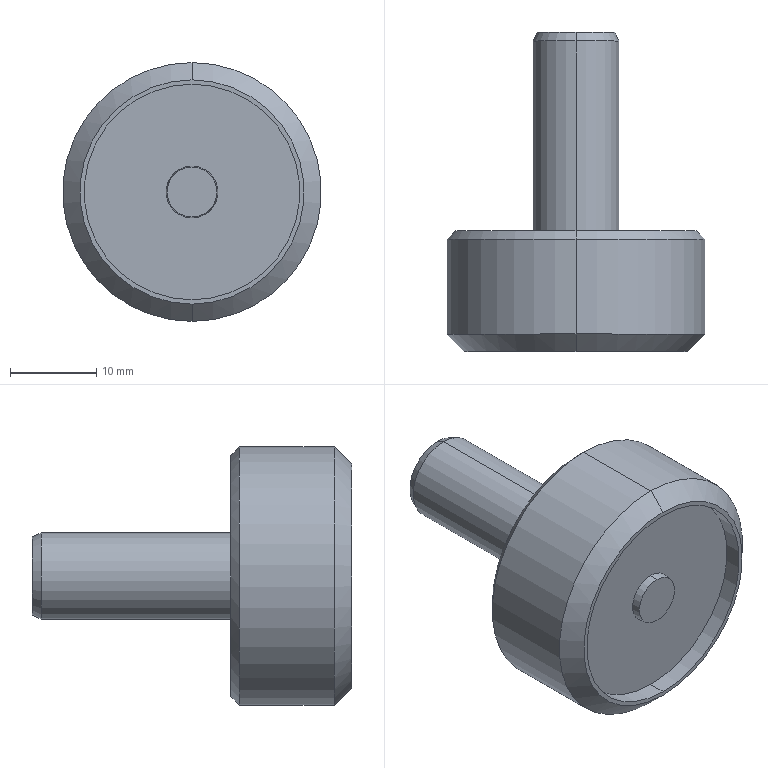Part | SolidWorks | features BaseBody 1 | 1 solid | 19 faces | box 30 x 37 x 30 mm | volume 10515 mm3 | cone 8 | cylinder 6 | plane 5 | commonest cylinder face diameters 10 x2 25 x2 30 x2
STEP:
#1=CARTESIAN_POINT('',(-257.5,37.,198.121));
#2=VERTEX_POINT('',#1);
#3=CARTESIAN_POINT('',(-257.5,37.,208.121));
#4=VERTEX_POINT('',#3);
#5=CARTESIAN_POINT('',(-257.5,37.,203.121));
#6=DIRECTION('',(0.,-1.,0.));
#7=DIRECTION('',(0.,0.,1.));
#8=AXIS2_PLACEMENT_3D('',#5,#6,#7);
#9=CIRCLE('',#8,5.);
#10=EDGE_CURVE('',#2,#4,#9,.T.);
#11=ORIENTED_EDGE('',*,*,#10,.F.);
#12=CARTESIAN_POINT('',(-257.5,59.,198.121));
#13=VERTEX_POINT('',#12);
#14=CARTESIAN_POINT('',(-257.5,60.,198.121));
#15=DIRECTION('',(0.,1.,0.));
#16=VECTOR('',#15,1000.);
#17=LINE('',#14,#16);
#18=EDGE_CURVE('',#2,#13,#17,.T.);
#19=ORIENTED_EDGE('',*,*,#18,.T.);
#20=CARTESIAN_POINT('',(-257.5,59.,208.121));
#21=VERTEX_POINT('',#20);
#22=CARTESIAN_POINT('',(-257.5,59.,203.121));
#23=DIRECTION('',(0.,-1.,0.));
#24=DIRECTION('',(0.,0.,1.));
#25=AXIS2_PLACEMENT_3D('',#22,#23,#24);
#26=CIRCLE('',#25,5.);
#27=EDGE_CURVE('',#13,#21,#26,.T.);
#28=ORIENTED_EDGE('',*,*,#27,.T.);
#29=CARTESIAN_POINT('',(-257.5,60.,208.121));
#30=DIRECTION('',(0.,1.,0.));
#31=VECTOR('',#30,1000.);
#32=LINE('',#29,#31);
#33=EDGE_CURVE('',#4,#21,#32,.T.);
#34=ORIENTED_EDGE('',*,*,#33,.F.);
#35=EDGE_LOOP('',(#11,#19,#28,#34));
#36=FACE_OUTER_BOUND('',#35,.T.);
#37=CARTESIAN_POINT('',(-257.5,60.,203.121));
#38=DIRECTION('',(0.,1.,0.));
#39=DIRECTION('',(0.,0.,1.));
#40=AXIS2_PLACEMENT_3D('',#37,#38,#39);
#41=CYLINDRICAL_SURFACE('',#40,5.);
#42=ADVANCED_FACE('',(#36),#41,.T.);
#43=CARTESIAN_POINT('',(-257.5,37.,217.121));
#44=VERTEX_POINT('',#43);
#45=CARTESIAN_POINT('',(-257.5,37.,189.121));
#46=VERTEX_POINT('',#45);
#47=CARTESIAN_POINT('',(-257.5,37.,203.121));
#48=DIRECTION('',(0.,1.,0.));
#49=DIRECTION('',(0.,0.,-1.));
#50=AXIS2_PLACEMENT_3D('',#47,#48,#49);
#51=CIRCLE('',#50,14.);
#52=EDGE_CURVE('',#44,#46,#51,.T.);
#53=ORIENTED_EDGE('',*,*,#52,.F.);
#54=CARTESIAN_POINT('',(-257.5,36.,218.121));
#55=VERTEX_POINT('',#54);
#56=CARTESIAN_POINT('',(-257.5,36.,218.121));
#57=DIRECTION('',(0.,-0.7071,0.7071));
#58=VECTOR('',#57,1000.);
#59=LINE('',#56,#58);
#60=EDGE_CURVE('',#44,#55,#59,.T.);
#61=ORIENTED_EDGE('',*,*,#60,.T.);
#62=CARTESIAN_POINT('',(-257.5,36.,188.121));
#63=VERTEX_POINT('',#62);
#64=CARTESIAN_POINT('',(-257.5,36.,203.121));
#65=DIRECTION('',(0.,1.,0.));
#66=DIRECTION('',(0.9739,0.,-0.227));
#67=AXIS2_PLACEMENT_3D('',#64,#65,#66);
#68=CIRCLE('',#67,15.);
#69=EDGE_CURVE('',#55,#63,#68,.T.);
#70=ORIENTED_EDGE('',*,*,#69,.T.);
#71=CARTESIAN_POINT('',(-257.5,36.,188.121));
#72=DIRECTION('',(0.,-0.7071,-0.7071));
#73=VECTOR('',#72,1000.);
#74=LINE('',#71,#73);
#75=EDGE_CURVE('',#46,#63,#74,.T.);
#76=ORIENTED_EDGE('',*,*,#75,.F.);
#77=EDGE_LOOP('',(#53,#61,#70,#76));
#78=FACE_OUTER_BOUND('',#77,.T.);
#79=CARTESIAN_POINT('',(-257.5,36.,203.121));
#80=DIRECTION('',(0.,-1.,0.));
#81=DIRECTION('',(0.,0.,-1.));
#82=AXIS2_PLACEMENT_3D('',#79,#80,#81);
#83=CONICAL_SURFACE('',#82,15.,0.7854);
#84=ADVANCED_FACE('',(#78),#83,.T.);
#85=CARTESIAN_POINT('',(-257.5,60.,198.587));
#86=VERTEX_POINT('',#85);
#87=CARTESIAN_POINT('',(-257.5,60.,207.655));
#88=VERTEX_POINT('',#87);
#89=CARTESIAN_POINT('',(-257.5,60.,203.121));
#90=DIRECTION('',(0.,-1.,0.));
#91=DIRECTION('',(0.,0.,-1.));
#92=AXIS2_PLACEMENT_3D('',#89,#90,#91);
#93=CIRCLE('',#92,4.534);
#94=EDGE_CURVE('',#86,#88,#93,.T.);
#95=ORIENTED_EDGE('',*,*,#94,.T.);
#96=CARTESIAN_POINT('',(-257.5,59.,208.121));
#97=DIRECTION('',(0.,-0.9063,0.4226));
#98=VECTOR('',#97,1000.);
#99=LINE('',#96,#98);
#100=EDGE_CURVE('',#88,#21,#99,.T.);
#101=ORIENTED_EDGE('',*,*,#100,.T.);
#102=ORIENTED_EDGE('',*,*,#27,.F.);
#103=CARTESIAN_POINT('',(-257.5,59.,198.121));
#104=DIRECTION('',(0.,-0.9063,-0.4226));
#105=VECTOR('',#104,1000.);
#106=LINE('',#103,#105);
#107=EDGE_CURVE('',#86,#13,#106,.T.);
#108=ORIENTED_EDGE('',*,*,#107,.F.);
#109=EDGE_LOOP('',(#95,#101,#102,#108));
#110=FACE_OUTER_BOUND('',#109,.T.);
#111=CARTESIAN_POINT('',(-257.5,59.,203.121));
#112=DIRECTION('',(0.,-1.,0.));
#113=DIRECTION('',(0.,0.,-1.));
#114=AXIS2_PLACEMENT_3D('',#111,#112,#113);
#115=CONICAL_SURFACE('',#114,5.,0.4363);
#116=ADVANCED_FACE('',(#110),#115,.T.);
#117=CARTESIAN_POINT('',(-257.5,25.,218.121));
#118=VERTEX_POINT('',#117);
#119=CARTESIAN_POINT('',(-257.5,25.,188.121));
#120=VERTEX_POINT('',#119);
#121=CARTESIAN_POINT('',(-257.5,25.,203.121));
#122=DIRECTION('',(0.,1.,0.));
#123=DIRECTION('',(0.,0.,1.));
#124=AXIS2_PLACEMENT_3D('',#121,#122,#123);
#125=CIRCLE('',#124,15.);
#126=EDGE_CURVE('',#118,#120,#125,.T.);
#127=ORIENTED_EDGE('',*,*,#126,.T.);
#128=CARTESIAN_POINT('',(-257.5,60.,188.121));
#129=DIRECTION('',(0.,1.,0.));
#130=VECTOR('',#129,1000.);
#131=LINE('',#128,#130);
#132=EDGE_CURVE('',#120,#63,#131,.T.);
#133=ORIENTED_EDGE('',*,*,#132,.T.);
#134=ORIENTED_EDGE('',*,*,#69,.F.);
#135=CARTESIAN_POINT('',(-257.5,60.,218.121));
#136=DIRECTION('',(0.,1.,0.));
#137=VECTOR('',#136,1000.);
#138=LINE('',#135,#137);
#139=EDGE_CURVE('',#118,#55,#138,.T.);
#140=ORIENTED_EDGE('',*,*,#139,.F.);
#141=EDGE_LOOP('',(#127,#133,#134,#140));
#142=FACE_OUTER_BOUND('',#141,.T.);
#143=CARTESIAN_POINT('',(-257.5,60.,203.121));
#144=DIRECTION('',(0.,1.,0.));
#145=DIRECTION('',(0.,0.,1.));
#146=AXIS2_PLACEMENT_3D('',#143,#144,#145);
#147=CYLINDRICAL_SURFACE('',#146,15.);
#148=ADVANCED_FACE('',(#142),#147,.T.);
#149=CARTESIAN_POINT('',(-257.5,23.,216.121));
#150=VERTEX_POINT('',#149);
#151=CARTESIAN_POINT('',(-257.5,23.,190.121));
#152=VERTEX_POINT('',#151);
#153=CARTESIAN_POINT('',(-257.5,23.,203.121));
#154=DIRECTION('',(0.,1.,0.));
#155=DIRECTION('',(0.,0.,1.));
#156=AXIS2_PLACEMENT_3D('',#153,#154,#155);
#157=CIRCLE('',#156,13.);
#158=EDGE_CURVE('',#150,#152,#157,.T.);
#159=ORIENTED_EDGE('',*,*,#158,.T.);
#160=CARTESIAN_POINT('',(-257.5,25.,188.121));
#161=DIRECTION('',(0.,0.7071,-0.7071));
#162=VECTOR('',#161,1000.);
#163=LINE('',#160,#162);
#164=EDGE_CURVE('',#152,#120,#163,.T.);
#165=ORIENTED_EDGE('',*,*,#164,.T.);
#166=ORIENTED_EDGE('',*,*,#126,.F.);
#167=CARTESIAN_POINT('',(-257.5,25.,218.121));
#168=DIRECTION('',(0.,0.7071,0.7071));
#169=VECTOR('',#168,1000.);
#170=LINE('',#167,#169);
#171=EDGE_CURVE('',#150,#118,#170,.T.);
#172=ORIENTED_EDGE('',*,*,#171,.F.);
#173=EDGE_LOOP('',(#159,#165,#166,#172));
#174=FACE_OUTER_BOUND('',#173,.T.);
#175=CARTESIAN_POINT('',(-257.5,25.,203.121));
#176=DIRECTION('',(0.,1.,0.));
#177=DIRECTION('',(0.,0.,1.));
#178=AXIS2_PLACEMENT_3D('',#175,#176,#177);
#179=CONICAL_SURFACE('',#178,15.,0.7854);
#180=ADVANCED_FACE('',(#174),#179,.T.);
#181=CARTESIAN_POINT('',(-257.5,25.,215.621));
#182=VERTEX_POINT('',#181);
#183=CARTESIAN_POINT('',(-257.5,25.,190.621));
#184=VERTEX_POINT('',#183);
#185=CARTESIAN_POINT('',(-257.5,25.,203.121));
#186=DIRECTION('',(0.,-1.,0.));
#187=DIRECTION('',(0.,0.,-1.));
#188=AXIS2_PLACEMENT_3D('',#185,#186,#187);
#189=CIRCLE('',#188,12.5);
#190=EDGE_CURVE('',#182,#184,#189,.T.);
#191=ORIENTED_EDGE('',*,*,#190,.F.);
#192=CARTESIAN_POINT('',(-257.5,23.,215.621));
#193=VERTEX_POINT('',#192);
#194=CARTESIAN_POINT('',(-257.5,24.,215.621));
#195=DIRECTION('',(0.,-1.,0.));
#196=VECTOR('',#195,1000.);
#197=LINE('',#194,#196);
#198=EDGE_CURVE('',#182,#193,#197,.T.);
#199=ORIENTED_EDGE('',*,*,#198,.T.);
#200=CARTESIAN_POINT('',(-257.5,23.,190.621));
#201=VERTEX_POINT('',#200);
#202=CARTESIAN_POINT('',(-257.5,23.,203.121));
#203=DIRECTION('',(0.,1.,0.));
#204=DIRECTION('',(0.,0.,-1.));
#205=AXIS2_PLACEMENT_3D('',#202,#203,#204);
#206=CIRCLE('',#205,12.5);
#207=EDGE_CURVE('',#201,#193,#206,.T.);
#208=ORIENTED_EDGE('',*,*,#207,.F.);
#209=CARTESIAN_POINT('',(-257.5,24.,190.621));
#210=DIRECTION('',(0.,-1.,0.));
#211=VECTOR('',#210,1000.);
#212=LINE('',#209,#211);
#213=EDGE_CURVE('',#184,#201,#212,.T.);
#214=ORIENTED_EDGE('',*,*,#213,.F.);
#215=EDGE_LOOP('',(#191,#199,#208,#214));
#216=FACE_OUTER_BOUND('',#215,.T.);
#217=CARTESIAN_POINT('',(-257.5,24.,203.121));
#218=DIRECTION('',(0.,-1.,0.));
#219=DIRECTION('',(0.,0.,-1.));
#220=AXIS2_PLACEMENT_3D('',#217,#218,#219);
#221=CYLINDRICAL_SURFACE('',#220,12.5);
#222=ADVANCED_FACE('',(#216),#221,.F.);
#223=CARTESIAN_POINT('',(-257.5,24.,206.016));
#224=VERTEX_POINT('',#223);
#225=CARTESIAN_POINT('',(-257.5,24.,200.226));
#226=VERTEX_POINT('',#225);
#227=CARTESIAN_POINT('',(-257.5,24.,203.121));
#228=DIRECTION('',(0.,1.,0.));
#229=DIRECTION('',(0.,0.,1.));
#230=AXIS2_PLACEMENT_3D('',#227,#228,#229);
#231=CIRCLE('',#230,2.895);
#232=EDGE_CURVE('',#224,#226,#231,.T.);
#233=ORIENTED_EDGE('',*,*,#232,.T.);
#234=CARTESIAN_POINT('',(-257.5,25.,200.121));
#235=VERTEX_POINT('',#234);
#236=CARTESIAN_POINT('',(-257.5,25.,200.121));
#237=DIRECTION('',(0.,0.9945,-0.1045));
#238=VECTOR('',#237,1000.);
#239=LINE('',#236,#238);
#240=EDGE_CURVE('',#226,#235,#239,.T.);
#241=ORIENTED_EDGE('',*,*,#240,.T.);
#242=CARTESIAN_POINT('',(-257.5,25.,206.121));
#243=VERTEX_POINT('',#242);
#244=CARTESIAN_POINT('',(-257.5,25.,203.121));
#245=DIRECTION('',(0.,1.,0.));
#246=DIRECTION('',(0.,0.,1.));
#247=AXIS2_PLACEMENT_3D('',#244,#245,#246);
#248=CIRCLE('',#247,3.);
#249=EDGE_CURVE('',#243,#235,#248,.T.);
#250=ORIENTED_EDGE('',*,*,#249,.F.);
#251=CARTESIAN_POINT('',(-257.5,25.,206.121));
#252=DIRECTION('',(0.,0.9945,0.1045));
#253=VECTOR('',#252,1000.);
#254=LINE('',#251,#253);
#255=EDGE_CURVE('',#224,#243,#254,.T.);
#256=ORIENTED_EDGE('',*,*,#255,.F.);
#257=EDGE_LOOP('',(#233,#241,#250,#256));
#258=FACE_OUTER_BOUND('',#257,.T.);
#259=CARTESIAN_POINT('',(-257.5,25.,203.121));
#260=DIRECTION('',(0.,1.,0.));
#261=DIRECTION('',(0.,0.,1.));
#262=AXIS2_PLACEMENT_3D('',#259,#260,#261);
#263=CONICAL_SURFACE('',#262,3.,0.1047);
#264=ADVANCED_FACE('',(#258),#263,.T.);
#265=CARTESIAN_POINT('',(-257.5,37.,203.121));
#266=DIRECTION('',(0.,-1.,0.));
#267=DIRECTION('',(0.,0.,1.));
#268=AXIS2_PLACEMENT_3D('',#265,#266,#267);
#269=CIRCLE('',#268,5.);
#270=EDGE_CURVE('',#4,#2,#269,.T.);
#271=ORIENTED_EDGE('',*,*,#270,.T.);
#272=ORIENTED_EDGE('',*,*,#10,.T.);
#273=EDGE_LOOP('',(#271,#272));
#274=FACE_BOUND('',#273,.T.);
#275=CARTESIAN_POINT('',(-257.5,37.,203.121));
#276=DIRECTION('',(0.,1.,0.));
#277=DIRECTION('',(0.,0.,-1.));
#278=AXIS2_PLACEMENT_3D('',#275,#276,#277);
#279=CIRCLE('',#278,14.);
#280=EDGE_CURVE('',#46,#44,#279,.T.);
#281=ORIENTED_EDGE('',*,*,#280,.T.);
#282=ORIENTED_EDGE('',*,*,#52,.T.);
#283=EDGE_LOOP('',(#281,#282));
#284=FACE_OUTER_BOUND('',#283,.T.);
#285=CARTESIAN_POINT('',(-272.108,37.,206.527));
#286=DIRECTION('',(0.,1.,0.));
#287=DIRECTION('',(0.,0.,1.));
#288=AXIS2_PLACEMENT_3D('',#285,#286,#287);
#289=PLANE('',#288);
#290=ADVANCED_FACE('',(#274,#284),#289,.T.);
#291=ORIENTED_EDGE('',*,*,#18,.F.);
#292=ORIENTED_EDGE('',*,*,#270,.F.);
#293=ORIENTED_EDGE('',*,*,#33,.T.);
#294=CARTESIAN_POINT('',(-257.5,59.,203.121));
#295=DIRECTION('',(0.,-1.,0.));
#296=DIRECTION('',(0.,0.,1.));
#297=AXIS2_PLACEMENT_3D('',#294,#295,#296);
#298=CIRCLE('',#297,5.);
#299=EDGE_CURVE('',#21,#13,#298,.T.);
#300=ORIENTED_EDGE('',*,*,#299,.T.);
#301=EDGE_LOOP('',(#291,#292,#293,#300));
#302=FACE_OUTER_BOUND('',#301,.T.);
#303=CARTESIAN_POINT('',(-257.5,60.,203.121));
#304=DIRECTION('',(0.,1.,0.));
#305=DIRECTION('',(0.,0.,1.));
#306=AXIS2_PLACEMENT_3D('',#303,#304,#305);
#307=CYLINDRICAL_SURFACE('',#306,5.);
#308=ADVANCED_FACE('',(#302),#307,.T.);
#309=ORIENTED_EDGE('',*,*,#60,.F.);
#310=ORIENTED_EDGE('',*,*,#280,.F.);
#311=ORIENTED_EDGE('',*,*,#75,.T.);
#312=CARTESIAN_POINT('',(-257.5,36.,203.121));
#313=DIRECTION('',(0.,1.,0.));
#314=DIRECTION('',(0.9739,0.,-0.227));
#315=AXIS2_PLACEMENT_3D('',#312,#313,#314);
#316=CIRCLE('',#315,15.);
#317=EDGE_CURVE('',#63,#55,#316,.T.);
#318=ORIENTED_EDGE('',*,*,#317,.T.);
#319=EDGE_LOOP('',(#309,#310,#311,#318));
#320=FACE_OUTER_BOUND('',#319,.T.);
#321=CARTESIAN_POINT('',(-257.5,36.,203.121));
#322=DIRECTION('',(0.,-1.,0.));
#323=DIRECTION('',(0.,0.,-1.));
#324=AXIS2_PLACEMENT_3D('',#321,#322,#323);
#325=CONICAL_SURFACE('',#324,15.,0.7854);
#326=ADVANCED_FACE('',(#320),#325,.T.);
#327=ORIENTED_EDGE('',*,*,#100,.F.);
#328=CARTESIAN_POINT('',(-257.5,60.,203.121));
#329=DIRECTION('',(0.,-1.,0.));
#330=DIRECTION('',(0.,0.,-1.));
#331=AXIS2_PLACEMENT_3D('',#328,#329,#330);
#332=CIRCLE('',#331,4.534);
#333=EDGE_CURVE('',#88,#86,#332,.T.);
#334=ORIENTED_EDGE('',*,*,#333,.T.);
#335=ORIENTED_EDGE('',*,*,#107,.T.);
#336=ORIENTED_EDGE('',*,*,#299,.F.);
#337=EDGE_LOOP('',(#327,#334,#335,#336));
#338=FACE_OUTER_BOUND('',#337,.T.);
#339=CARTESIAN_POINT('',(-257.5,59.,203.121));
#340=DIRECTION('',(0.,-1.,0.));
#341=DIRECTION('',(0.,0.,-1.));
#342=AXIS2_PLACEMENT_3D('',#339,#340,#341);
#343=CONICAL_SURFACE('',#342,5.,0.4363);
#344=ADVANCED_FACE('',(#338),#343,.T.);
#345=ORIENTED_EDGE('',*,*,#132,.F.);
#346=CARTESIAN_POINT('',(-257.5,25.,203.121));
#347=DIRECTION('',(0.,1.,0.));
#348=DIRECTION('',(0.,0.,1.));
#349=AXIS2_PLACEMENT_3D('',#346,#347,#348);
#350=CIRCLE('',#349,15.);
#351=EDGE_CURVE('',#120,#118,#350,.T.);
#352=ORIENTED_EDGE('',*,*,#351,.T.);
#353=ORIENTED_EDGE('',*,*,#139,.T.);
#354=ORIENTED_EDGE('',*,*,#317,.F.);
#355=EDGE_LOOP('',(#345,#352,#353,#354));
#356=FACE_OUTER_BOUND('',#355,.T.);
#357=CARTESIAN_POINT('',(-257.5,60.,203.121));
#358=DIRECTION('',(0.,1.,0.));
#359=DIRECTION('',(0.,0.,1.));
#360=AXIS2_PLACEMENT_3D('',#357,#358,#359);
#361=CYLINDRICAL_SURFACE('',#360,15.);
#362=ADVANCED_FACE('',(#356),#361,.T.);
#363=ORIENTED_EDGE('',*,*,#94,.F.);
#364=ORIENTED_EDGE('',*,*,#333,.F.);
#365=EDGE_LOOP('',(#363,#364));
#366=FACE_OUTER_BOUND('',#365,.T.);
#367=CARTESIAN_POINT('',(-262.369,60.,204.256));
#368=DIRECTION('',(0.,1.,0.));
#369=DIRECTION('',(0.,0.,1.));
#370=AXIS2_PLACEMENT_3D('',#367,#368,#369);
#371=PLANE('',#370);
#372=ADVANCED_FACE('',(#366),#371,.T.);
#373=ORIENTED_EDGE('',*,*,#164,.F.);
#374=CARTESIAN_POINT('',(-257.5,23.,203.121));
#375=DIRECTION('',(0.,1.,0.));
#376=DIRECTION('',(0.,0.,1.));
#377=AXIS2_PLACEMENT_3D('',#374,#375,#376);
#378=CIRCLE('',#377,13.);
#379=EDGE_CURVE('',#152,#150,#378,.T.);
#380=ORIENTED_EDGE('',*,*,#379,.T.);
#381=ORIENTED_EDGE('',*,*,#171,.T.);
#382=ORIENTED_EDGE('',*,*,#351,.F.);
#383=EDGE_LOOP('',(#373,#380,#381,#382));
#384=FACE_OUTER_BOUND('',#383,.T.);
#385=CARTESIAN_POINT('',(-257.5,25.,203.121));
#386=DIRECTION('',(0.,1.,0.));
#387=DIRECTION('',(0.,0.,1.));
#388=AXIS2_PLACEMENT_3D('',#385,#386,#387);
#389=CONICAL_SURFACE('',#388,15.,0.7854);
#390=ADVANCED_FACE('',(#384),#389,.T.);
#391=ORIENTED_EDGE('',*,*,#158,.F.);
#392=ORIENTED_EDGE('',*,*,#379,.F.);
#393=EDGE_LOOP('',(#391,#392));
#394=FACE_OUTER_BOUND('',#393,.T.);
#395=ORIENTED_EDGE('',*,*,#207,.T.);
#396=CARTESIAN_POINT('',(-257.5,23.,203.121));
#397=DIRECTION('',(0.,1.,0.));
#398=DIRECTION('',(0.,0.,-1.));
#399=AXIS2_PLACEMENT_3D('',#396,#397,#398);
#400=CIRCLE('',#399,12.5);
#401=EDGE_CURVE('',#193,#201,#400,.T.);
#402=ORIENTED_EDGE('',*,*,#401,.T.);
#403=EDGE_LOOP('',(#395,#402));
#404=FACE_BOUND('',#403,.T.);
#405=CARTESIAN_POINT('',(-257.5,23.,203.121));
#406=DIRECTION('',(0.,-1.,0.));
#407=DIRECTION('',(0.,0.,-1.));
#408=AXIS2_PLACEMENT_3D('',#405,#406,#407);
#409=PLANE('',#408);
#410=ADVANCED_FACE('',(#394,#404),#409,.T.);
#411=ORIENTED_EDGE('',*,*,#198,.F.);
#412=CARTESIAN_POINT('',(-257.5,25.,203.121));
#413=DIRECTION('',(0.,-1.,0.));
#414=DIRECTION('',(0.,0.,-1.));
#415=AXIS2_PLACEMENT_3D('',#412,#413,#414);
#416=CIRCLE('',#415,12.5);
#417=EDGE_CURVE('',#184,#182,#416,.T.);
#418=ORIENTED_EDGE('',*,*,#417,.F.);
#419=ORIENTED_EDGE('',*,*,#213,.T.);
#420=ORIENTED_EDGE('',*,*,#401,.F.);
#421=EDGE_LOOP('',(#411,#418,#419,#420));
#422=FACE_OUTER_BOUND('',#421,.T.);
#423=CARTESIAN_POINT('',(-257.5,24.,203.121));
#424=DIRECTION('',(0.,-1.,0.));
#425=DIRECTION('',(0.,0.,-1.));
#426=AXIS2_PLACEMENT_3D('',#423,#424,#425);
#427=CYLINDRICAL_SURFACE('',#426,12.5);
#428=ADVANCED_FACE('',(#422),#427,.F.);
#429=ORIENTED_EDGE('',*,*,#249,.T.);
#430=CARTESIAN_POINT('',(-257.5,25.,203.121));
#431=DIRECTION('',(0.,1.,0.));
#432=DIRECTION('',(0.,0.,1.));
#433=AXIS2_PLACEMENT_3D('',#430,#431,#432);
#434=CIRCLE('',#433,3.);
#435=EDGE_CURVE('',#235,#243,#434,.T.);
#436=ORIENTED_EDGE('',*,*,#435,.T.);
#437=EDGE_LOOP('',(#429,#436));
#438=FACE_BOUND('',#437,.T.);
#439=ORIENTED_EDGE('',*,*,#417,.T.);
#440=ORIENTED_EDGE('',*,*,#190,.T.);
#441=EDGE_LOOP('',(#439,#440));
#442=FACE_OUTER_BOUND('',#441,.T.);
#443=CARTESIAN_POINT('',(-257.5,25.,203.121));
#444=DIRECTION('',(0.,-1.,0.));
#445=DIRECTION('',(0.,0.,-1.));
#446=AXIS2_PLACEMENT_3D('',#443,#444,#445);
#447=PLANE('',#446);
#448=ADVANCED_FACE('',(#438,#442),#447,.T.);
#449=ORIENTED_EDGE('',*,*,#240,.F.);
#450=CARTESIAN_POINT('',(-257.5,24.,203.121));
#451=DIRECTION('',(0.,1.,0.));
#452=DIRECTION('',(0.,0.,1.));
#453=AXIS2_PLACEMENT_3D('',#450,#451,#452);
#454=CIRCLE('',#453,2.895);
#455=EDGE_CURVE('',#226,#224,#454,.T.);
#456=ORIENTED_EDGE('',*,*,#455,.T.);
#457=ORIENTED_EDGE('',*,*,#255,.T.);
#458=ORIENTED_EDGE('',*,*,#435,.F.);
#459=EDGE_LOOP('',(#449,#456,#457,#458));
#460=FACE_OUTER_BOUND('',#459,.T.);
#461=CARTESIAN_POINT('',(-257.5,25.,203.121));
#462=DIRECTION('',(0.,1.,0.));
#463=DIRECTION('',(0.,0.,1.));
#464=AXIS2_PLACEMENT_3D('',#461,#462,#463);
#465=CONICAL_SURFACE('',#464,3.,0.1047);
#466=ADVANCED_FACE('',(#460),#465,.T.);
#467=ORIENTED_EDGE('',*,*,#232,.F.);
#468=ORIENTED_EDGE('',*,*,#455,.F.);
#469=EDGE_LOOP('',(#467,#468));
#470=FACE_OUTER_BOUND('',#469,.T.);
#471=CARTESIAN_POINT('',(-257.5,24.,203.121));
#472=DIRECTION('',(0.,-1.,0.));
#473=DIRECTION('',(0.,0.,-1.));
#474=AXIS2_PLACEMENT_3D('',#471,#472,#473);
#475=PLANE('',#474);
#476=ADVANCED_FACE('',(#470),#475,.T.);
#477=CLOSED_SHELL('',(#42,#84,#116,#148,#180,#222,#264,#290,#308,#326,#344,#362,#372,#390,#410,#428,#448,#466,#476));
#478=MANIFOLD_SOLID_BREP('',#477);
#479=CARTESIAN_POINT('',(0.,0.,0.));
#480=DIRECTION('',(0.,0.,1.));
#481=DIRECTION('',(1.,0.,0.));
#482=AXIS2_PLACEMENT_3D('',#479,#480,#481);
#483=(LENGTH_UNIT()NAMED_UNIT(*)SI_UNIT(.MILLI.,.METRE.));
#484=UNCERTAINTY_MEASURE_WITH_UNIT(LENGTH_MEASURE(0.00001),#483,'','');
#485=(NAMED_UNIT(*)PLANE_ANGLE_UNIT()SI_UNIT($,.RADIAN.));
#486=(NAMED_UNIT(*)SI_UNIT($,.STERADIAN.)SOLID_ANGLE_UNIT());
#487=(GEOMETRIC_REPRESENTATION_CONTEXT(3)GLOBAL_UNCERTAINTY_ASSIGNED_CONTEXT((#484))GLOBAL_UNIT_ASSIGNED_CONTEXT((#483,#485,#486))REPRESENTATION_CONTEXT('',''));
#488=ADVANCED_BREP_SHAPE_REPRESENTATION('',(#478,#482),#487);